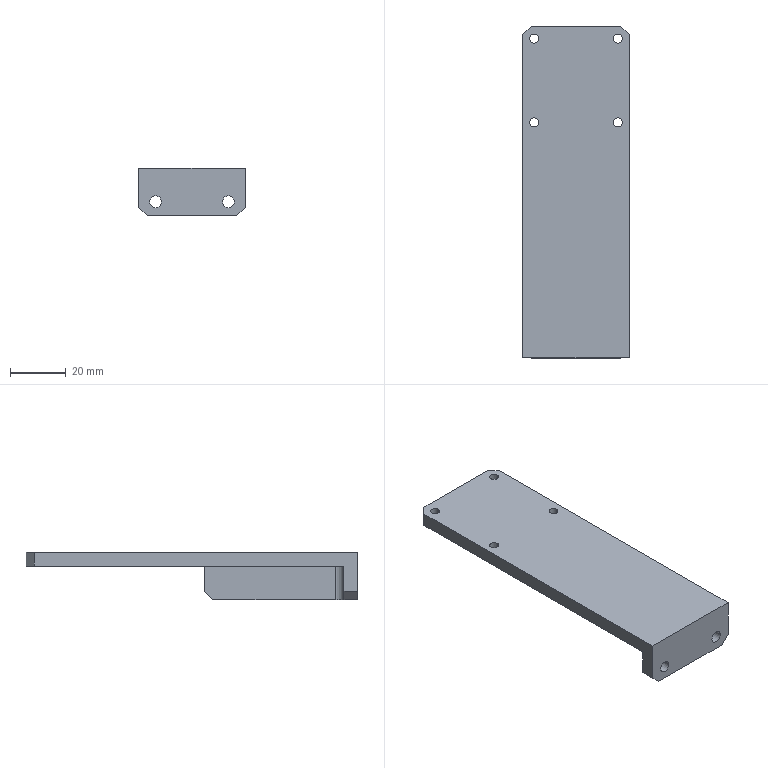Part | NX | 1 solid | 31 faces | box 38.1 x 118.8 x 17 mm | volume 29338 mm3 | plane 17 | cylinder 14 | commonest cylinder face diameters 3.2 x8 4.2 x4 6 x2
STEP:
#1=CARTESIAN_POINT('',(-13.4,24.9,-5.));
#2=VERTEX_POINT('',#1);
#3=CARTESIAN_POINT('',(-16.6,24.9,-5.));
#4=VERTEX_POINT('',#3);
#5=CARTESIAN_POINT('',(-15.,24.9,-5.));
#6=DIRECTION('',(0.,0.,-1.));
#7=DIRECTION('',(-1.,0.,0.));
#8=AXIS2_PLACEMENT_3D('',#5,#6,#7);
#9=CIRCLE('',#8,1.6);
#10=EDGE_CURVE('',#2,#4,#9,.T.);
#11=ORIENTED_EDGE('',*,*,#10,.T.);
#12=CARTESIAN_POINT('',(-16.6,24.9,0.));
#13=VERTEX_POINT('',#12);
#14=CARTESIAN_POINT('',(-16.6,24.9,-17.));
#15=DIRECTION('',(0.,0.,1.));
#16=VECTOR('',#15,1000.);
#17=LINE('',#14,#16);
#18=EDGE_CURVE('',#4,#13,#17,.T.);
#19=ORIENTED_EDGE('',*,*,#18,.T.);
#20=CARTESIAN_POINT('',(-13.4,24.9,0.));
#21=VERTEX_POINT('',#20);
#22=CARTESIAN_POINT('',(-15.,24.9,0.));
#23=DIRECTION('',(0.,0.,1.));
#24=DIRECTION('',(1.,0.,0.));
#25=AXIS2_PLACEMENT_3D('',#22,#23,#24);
#26=CIRCLE('',#25,1.6);
#27=EDGE_CURVE('',#13,#21,#26,.T.);
#28=ORIENTED_EDGE('',*,*,#27,.T.);
#29=CARTESIAN_POINT('',(-13.4,24.9,-17.));
#30=DIRECTION('',(0.,0.,1.));
#31=VECTOR('',#30,1000.);
#32=LINE('',#29,#31);
#33=EDGE_CURVE('',#2,#21,#32,.T.);
#34=ORIENTED_EDGE('',*,*,#33,.F.);
#35=EDGE_LOOP('',(#11,#19,#28,#34));
#36=FACE_BOUND('',#35,.T.);
#37=CARTESIAN_POINT('',(-15.,24.9,-17.));
#38=DIRECTION('',(0.,0.,1.));
#39=DIRECTION('',(-1.,0.,0.));
#40=AXIS2_PLACEMENT_3D('',#37,#38,#39);
#41=CYLINDRICAL_SURFACE('',#40,1.6);
#42=ADVANCED_FACE('',(#36),#41,.F.);
#43=CARTESIAN_POINT('',(16.6,24.9,-5.));
#44=VERTEX_POINT('',#43);
#45=CARTESIAN_POINT('',(13.4,24.9,-5.));
#46=VERTEX_POINT('',#45);
#47=CARTESIAN_POINT('',(15.,24.9,-5.));
#48=DIRECTION('',(0.,0.,-1.));
#49=DIRECTION('',(-1.,0.,0.));
#50=AXIS2_PLACEMENT_3D('',#47,#48,#49);
#51=CIRCLE('',#50,1.6);
#52=EDGE_CURVE('',#44,#46,#51,.T.);
#53=ORIENTED_EDGE('',*,*,#52,.T.);
#54=CARTESIAN_POINT('',(13.4,24.9,0.));
#55=VERTEX_POINT('',#54);
#56=CARTESIAN_POINT('',(13.4,24.9,-17.));
#57=DIRECTION('',(0.,0.,1.));
#58=VECTOR('',#57,1000.);
#59=LINE('',#56,#58);
#60=EDGE_CURVE('',#46,#55,#59,.T.);
#61=ORIENTED_EDGE('',*,*,#60,.T.);
#62=CARTESIAN_POINT('',(16.6,24.9,0.));
#63=VERTEX_POINT('',#62);
#64=CARTESIAN_POINT('',(15.,24.9,0.));
#65=DIRECTION('',(0.,0.,1.));
#66=DIRECTION('',(1.,0.,0.));
#67=AXIS2_PLACEMENT_3D('',#64,#65,#66);
#68=CIRCLE('',#67,1.6);
#69=EDGE_CURVE('',#55,#63,#68,.T.);
#70=ORIENTED_EDGE('',*,*,#69,.T.);
#71=CARTESIAN_POINT('',(16.6,24.9,-17.));
#72=DIRECTION('',(0.,0.,1.));
#73=VECTOR('',#72,1000.);
#74=LINE('',#71,#73);
#75=EDGE_CURVE('',#44,#63,#74,.T.);
#76=ORIENTED_EDGE('',*,*,#75,.F.);
#77=EDGE_LOOP('',(#53,#61,#70,#76));
#78=FACE_BOUND('',#77,.T.);
#79=CARTESIAN_POINT('',(15.,24.9,-17.));
#80=DIRECTION('',(0.,0.,1.));
#81=DIRECTION('',(-1.,0.,0.));
#82=AXIS2_PLACEMENT_3D('',#79,#80,#81);
#83=CYLINDRICAL_SURFACE('',#82,1.6);
#84=ADVANCED_FACE('',(#78),#83,.F.);
#85=CARTESIAN_POINT('',(16.6,54.9,-5.));
#86=VERTEX_POINT('',#85);
#87=CARTESIAN_POINT('',(13.4,54.9,-5.));
#88=VERTEX_POINT('',#87);
#89=CARTESIAN_POINT('',(15.,54.9,-5.));
#90=DIRECTION('',(0.,0.,-1.));
#91=DIRECTION('',(-1.,0.,0.));
#92=AXIS2_PLACEMENT_3D('',#89,#90,#91);
#93=CIRCLE('',#92,1.6);
#94=EDGE_CURVE('',#86,#88,#93,.T.);
#95=ORIENTED_EDGE('',*,*,#94,.T.);
#96=CARTESIAN_POINT('',(13.4,54.9,0.));
#97=VERTEX_POINT('',#96);
#98=CARTESIAN_POINT('',(13.4,54.9,-17.));
#99=DIRECTION('',(0.,0.,1.));
#100=VECTOR('',#99,1000.);
#101=LINE('',#98,#100);
#102=EDGE_CURVE('',#88,#97,#101,.T.);
#103=ORIENTED_EDGE('',*,*,#102,.T.);
#104=CARTESIAN_POINT('',(16.6,54.9,0.));
#105=VERTEX_POINT('',#104);
#106=CARTESIAN_POINT('',(15.,54.9,0.));
#107=DIRECTION('',(0.,0.,1.));
#108=DIRECTION('',(1.,0.,0.));
#109=AXIS2_PLACEMENT_3D('',#106,#107,#108);
#110=CIRCLE('',#109,1.6);
#111=EDGE_CURVE('',#97,#105,#110,.T.);
#112=ORIENTED_EDGE('',*,*,#111,.T.);
#113=CARTESIAN_POINT('',(16.6,54.9,-17.));
#114=DIRECTION('',(0.,0.,1.));
#115=VECTOR('',#114,1000.);
#116=LINE('',#113,#115);
#117=EDGE_CURVE('',#86,#105,#116,.T.);
#118=ORIENTED_EDGE('',*,*,#117,.F.);
#119=EDGE_LOOP('',(#95,#103,#112,#118));
#120=FACE_BOUND('',#119,.T.);
#121=CARTESIAN_POINT('',(15.,54.9,-17.));
#122=DIRECTION('',(0.,0.,1.));
#123=DIRECTION('',(-1.,0.,0.));
#124=AXIS2_PLACEMENT_3D('',#121,#122,#123);
#125=CYLINDRICAL_SURFACE('',#124,1.6);
#126=ADVANCED_FACE('',(#120),#125,.F.);
#127=CARTESIAN_POINT('',(-13.4,54.9,-5.));
#128=VERTEX_POINT('',#127);
#129=CARTESIAN_POINT('',(-16.6,54.9,-5.));
#130=VERTEX_POINT('',#129);
#131=CARTESIAN_POINT('',(-15.,54.9,-5.));
#132=DIRECTION('',(0.,0.,-1.));
#133=DIRECTION('',(-1.,0.,0.));
#134=AXIS2_PLACEMENT_3D('',#131,#132,#133);
#135=CIRCLE('',#134,1.6);
#136=EDGE_CURVE('',#128,#130,#135,.T.);
#137=ORIENTED_EDGE('',*,*,#136,.T.);
#138=CARTESIAN_POINT('',(-16.6,54.9,0.));
#139=VERTEX_POINT('',#138);
#140=CARTESIAN_POINT('',(-16.6,54.9,-17.));
#141=DIRECTION('',(0.,0.,1.));
#142=VECTOR('',#141,1000.);
#143=LINE('',#140,#142);
#144=EDGE_CURVE('',#130,#139,#143,.T.);
#145=ORIENTED_EDGE('',*,*,#144,.T.);
#146=CARTESIAN_POINT('',(-13.4,54.9,0.));
#147=VERTEX_POINT('',#146);
#148=CARTESIAN_POINT('',(-15.,54.9,0.));
#149=DIRECTION('',(0.,0.,1.));
#150=DIRECTION('',(1.,0.,0.));
#151=AXIS2_PLACEMENT_3D('',#148,#149,#150);
#152=CIRCLE('',#151,1.6);
#153=EDGE_CURVE('',#139,#147,#152,.T.);
#154=ORIENTED_EDGE('',*,*,#153,.T.);
#155=CARTESIAN_POINT('',(-13.4,54.9,-17.));
#156=DIRECTION('',(0.,0.,1.));
#157=VECTOR('',#156,1000.);
#158=LINE('',#155,#157);
#159=EDGE_CURVE('',#128,#147,#158,.T.);
#160=ORIENTED_EDGE('',*,*,#159,.F.);
#161=EDGE_LOOP('',(#137,#145,#154,#160));
#162=FACE_BOUND('',#161,.T.);
#163=CARTESIAN_POINT('',(-15.,54.9,-17.));
#164=DIRECTION('',(0.,0.,1.));
#165=DIRECTION('',(-1.,0.,0.));
#166=AXIS2_PLACEMENT_3D('',#163,#164,#165);
#167=CYLINDRICAL_SURFACE('',#166,1.6);
#168=ADVANCED_FACE('',(#162),#167,.F.);
#169=CARTESIAN_POINT('',(-10.9,-59.4,-12.));
#170=VERTEX_POINT('',#169);
#171=CARTESIAN_POINT('',(-15.1,-59.4,-12.));
#172=VERTEX_POINT('',#171);
#173=CARTESIAN_POINT('',(-13.,-59.4,-12.));
#174=DIRECTION('',(0.,1.,0.));
#175=DIRECTION('',(-1.,0.,0.));
#176=AXIS2_PLACEMENT_3D('',#173,#174,#175);
#177=CIRCLE('',#176,2.1);
#178=EDGE_CURVE('',#170,#172,#177,.T.);
#179=ORIENTED_EDGE('',*,*,#178,.F.);
#180=CARTESIAN_POINT('',(-10.9,-54.4,-12.));
#181=VERTEX_POINT('',#180);
#182=CARTESIAN_POINT('',(-10.9,-59.4,-12.));
#183=DIRECTION('',(0.,1.,0.));
#184=VECTOR('',#183,1000.);
#185=LINE('',#182,#184);
#186=EDGE_CURVE('',#170,#181,#185,.T.);
#187=ORIENTED_EDGE('',*,*,#186,.T.);
#188=CARTESIAN_POINT('',(-15.1,-54.4,-12.));
#189=VERTEX_POINT('',#188);
#190=CARTESIAN_POINT('',(-13.,-54.4,-12.));
#191=DIRECTION('',(0.,1.,0.));
#192=DIRECTION('',(-1.,0.,0.));
#193=AXIS2_PLACEMENT_3D('',#190,#191,#192);
#194=CIRCLE('',#193,2.1);
#195=EDGE_CURVE('',#181,#189,#194,.T.);
#196=ORIENTED_EDGE('',*,*,#195,.T.);
#197=CARTESIAN_POINT('',(-15.1,-59.4,-12.));
#198=DIRECTION('',(0.,1.,0.));
#199=VECTOR('',#198,1000.);
#200=LINE('',#197,#199);
#201=EDGE_CURVE('',#172,#189,#200,.T.);
#202=ORIENTED_EDGE('',*,*,#201,.F.);
#203=EDGE_LOOP('',(#179,#187,#196,#202));
#204=FACE_BOUND('',#203,.T.);
#205=CARTESIAN_POINT('',(-13.,-59.4,-12.));
#206=DIRECTION('',(0.,1.,0.));
#207=DIRECTION('',(1.,0.,0.));
#208=AXIS2_PLACEMENT_3D('',#205,#206,#207);
#209=CYLINDRICAL_SURFACE('',#208,2.1);
#210=ADVANCED_FACE('',(#204),#209,.F.);
#211=CARTESIAN_POINT('',(15.1,-59.4,-12.));
#212=VERTEX_POINT('',#211);
#213=CARTESIAN_POINT('',(10.9,-59.4,-12.));
#214=VERTEX_POINT('',#213);
#215=CARTESIAN_POINT('',(13.,-59.4,-12.));
#216=DIRECTION('',(0.,1.,0.));
#217=DIRECTION('',(-1.,0.,0.));
#218=AXIS2_PLACEMENT_3D('',#215,#216,#217);
#219=CIRCLE('',#218,2.1);
#220=EDGE_CURVE('',#212,#214,#219,.T.);
#221=ORIENTED_EDGE('',*,*,#220,.F.);
#222=CARTESIAN_POINT('',(15.1,-54.4,-12.));
#223=VERTEX_POINT('',#222);
#224=CARTESIAN_POINT('',(15.1,-59.4,-12.));
#225=DIRECTION('',(0.,1.,0.));
#226=VECTOR('',#225,1000.);
#227=LINE('',#224,#226);
#228=EDGE_CURVE('',#212,#223,#227,.T.);
#229=ORIENTED_EDGE('',*,*,#228,.T.);
#230=CARTESIAN_POINT('',(10.9,-54.4,-12.));
#231=VERTEX_POINT('',#230);
#232=CARTESIAN_POINT('',(13.,-54.4,-12.));
#233=DIRECTION('',(0.,1.,0.));
#234=DIRECTION('',(-1.,0.,0.));
#235=AXIS2_PLACEMENT_3D('',#232,#233,#234);
#236=CIRCLE('',#235,2.1);
#237=EDGE_CURVE('',#223,#231,#236,.T.);
#238=ORIENTED_EDGE('',*,*,#237,.T.);
#239=CARTESIAN_POINT('',(10.9,-59.4,-12.));
#240=DIRECTION('',(0.,1.,0.));
#241=VECTOR('',#240,1000.);
#242=LINE('',#239,#241);
#243=EDGE_CURVE('',#214,#231,#242,.T.);
#244=ORIENTED_EDGE('',*,*,#243,.F.);
#245=EDGE_LOOP('',(#221,#229,#238,#244));
#246=FACE_BOUND('',#245,.T.);
#247=CARTESIAN_POINT('',(13.,-59.4,-12.));
#248=DIRECTION('',(0.,1.,0.));
#249=DIRECTION('',(1.,0.,0.));
#250=AXIS2_PLACEMENT_3D('',#247,#248,#249);
#251=CYLINDRICAL_SURFACE('',#250,2.1);
#252=ADVANCED_FACE('',(#246),#251,.F.);
#253=ORIENTED_EDGE('',*,*,#10,.F.);
#254=CARTESIAN_POINT('',(-15.,24.9,-5.));
#255=DIRECTION('',(0.,0.,-1.));
#256=DIRECTION('',(-1.,0.,0.));
#257=AXIS2_PLACEMENT_3D('',#254,#255,#256);
#258=CIRCLE('',#257,1.6);
#259=EDGE_CURVE('',#4,#2,#258,.T.);
#260=ORIENTED_EDGE('',*,*,#259,.F.);
#261=EDGE_LOOP('',(#253,#260));
#262=FACE_BOUND('',#261,.T.);
#263=ORIENTED_EDGE('',*,*,#52,.F.);
#264=CARTESIAN_POINT('',(15.,24.9,-5.));
#265=DIRECTION('',(0.,0.,-1.));
#266=DIRECTION('',(-1.,0.,0.));
#267=AXIS2_PLACEMENT_3D('',#264,#265,#266);
#268=CIRCLE('',#267,1.6);
#269=EDGE_CURVE('',#46,#44,#268,.T.);
#270=ORIENTED_EDGE('',*,*,#269,.F.);
#271=EDGE_LOOP('',(#263,#270));
#272=FACE_BOUND('',#271,.T.);
#273=ORIENTED_EDGE('',*,*,#94,.F.);
#274=CARTESIAN_POINT('',(15.,54.9,-5.));
#275=DIRECTION('',(0.,0.,-1.));
#276=DIRECTION('',(-1.,0.,0.));
#277=AXIS2_PLACEMENT_3D('',#274,#275,#276);
#278=CIRCLE('',#277,1.6);
#279=EDGE_CURVE('',#88,#86,#278,.T.);
#280=ORIENTED_EDGE('',*,*,#279,.F.);
#281=EDGE_LOOP('',(#273,#280));
#282=FACE_BOUND('',#281,.T.);
#283=ORIENTED_EDGE('',*,*,#136,.F.);
#284=CARTESIAN_POINT('',(-15.,54.9,-5.));
#285=DIRECTION('',(0.,0.,-1.));
#286=DIRECTION('',(-1.,0.,0.));
#287=AXIS2_PLACEMENT_3D('',#284,#285,#286);
#288=CIRCLE('',#287,1.6);
#289=EDGE_CURVE('',#130,#128,#288,.T.);
#290=ORIENTED_EDGE('',*,*,#289,.F.);
#291=EDGE_LOOP('',(#283,#290));
#292=FACE_BOUND('',#291,.T.);
#293=CARTESIAN_POINT('',(-4.,-51.4,-5.));
#294=VERTEX_POINT('',#293);
#295=CARTESIAN_POINT('',(-4.,-4.4,-5.));
#296=VERTEX_POINT('',#295);
#297=CARTESIAN_POINT('',(-4.,-54.4,-5.));
#298=DIRECTION('',(0.,1.,0.));
#299=VECTOR('',#298,1000.);
#300=LINE('',#297,#299);
#301=EDGE_CURVE('',#294,#296,#300,.T.);
#302=ORIENTED_EDGE('',*,*,#301,.F.);
#303=CARTESIAN_POINT('',(-7.,-54.4,-5.));
#304=VERTEX_POINT('',#303);
#305=CARTESIAN_POINT('',(-7.,-51.4,-5.));
#306=DIRECTION('',(0.,0.,-1.));
#307=DIRECTION('',(-1.,0.,0.));
#308=AXIS2_PLACEMENT_3D('',#305,#306,#307);
#309=CIRCLE('',#308,3.);
#310=EDGE_CURVE('',#294,#304,#309,.T.);
#311=ORIENTED_EDGE('',*,*,#310,.T.);
#312=CARTESIAN_POINT('',(-19.05,-54.4,-5.));
#313=VERTEX_POINT('',#312);
#314=CARTESIAN_POINT('',(-19.05,-54.4,-5.));
#315=DIRECTION('',(1.,0.,0.));
#316=VECTOR('',#315,1000.);
#317=LINE('',#314,#316);
#318=EDGE_CURVE('',#313,#304,#317,.T.);
#319=ORIENTED_EDGE('',*,*,#318,.F.);
#320=CARTESIAN_POINT('',(-19.05,56.4,-5.));
#321=VERTEX_POINT('',#320);
#322=CARTESIAN_POINT('',(-19.05,-59.4,-5.));
#323=DIRECTION('',(0.,-1.,0.));
#324=VECTOR('',#323,1000.);
#325=LINE('',#322,#324);
#326=EDGE_CURVE('',#321,#313,#325,.T.);
#327=ORIENTED_EDGE('',*,*,#326,.F.);
#328=CARTESIAN_POINT('',(-16.05,59.4,-5.));
#329=VERTEX_POINT('',#328);
#330=CARTESIAN_POINT('',(-76.95,-1.5,-5.));
#331=DIRECTION('',(0.7071,0.7071,0.));
#332=VECTOR('',#331,1000.);
#333=LINE('',#330,#332);
#334=EDGE_CURVE('',#321,#329,#333,.T.);
#335=ORIENTED_EDGE('',*,*,#334,.T.);
#336=CARTESIAN_POINT('',(16.05,59.4,-5.));
#337=VERTEX_POINT('',#336);
#338=CARTESIAN_POINT('',(-19.05,59.4,-5.));
#339=DIRECTION('',(-1.,0.,0.));
#340=VECTOR('',#339,1000.);
#341=LINE('',#338,#340);
#342=EDGE_CURVE('',#337,#329,#341,.T.);
#343=ORIENTED_EDGE('',*,*,#342,.F.);
#344=CARTESIAN_POINT('',(19.05,56.4,-5.));
#345=VERTEX_POINT('',#344);
#346=CARTESIAN_POINT('',(57.9,17.55,-5.));
#347=DIRECTION('',(0.7071,-0.7071,0.));
#348=VECTOR('',#347,1000.);
#349=LINE('',#346,#348);
#350=EDGE_CURVE('',#337,#345,#349,.T.);
#351=ORIENTED_EDGE('',*,*,#350,.T.);
#352=CARTESIAN_POINT('',(19.05,-54.4,-5.));
#353=VERTEX_POINT('',#352);
#354=CARTESIAN_POINT('',(19.05,-59.4,-5.));
#355=DIRECTION('',(0.,1.,0.));
#356=VECTOR('',#355,1000.);
#357=LINE('',#354,#356);
#358=EDGE_CURVE('',#353,#345,#357,.T.);
#359=ORIENTED_EDGE('',*,*,#358,.F.);
#360=CARTESIAN_POINT('',(7.,-54.4,-5.));
#361=VERTEX_POINT('',#360);
#362=CARTESIAN_POINT('',(-19.05,-54.4,-5.));
#363=DIRECTION('',(1.,0.,0.));
#364=VECTOR('',#363,1000.);
#365=LINE('',#362,#364);
#366=EDGE_CURVE('',#361,#353,#365,.T.);
#367=ORIENTED_EDGE('',*,*,#366,.F.);
#368=CARTESIAN_POINT('',(4.,-51.4,-5.));
#369=VERTEX_POINT('',#368);
#370=CARTESIAN_POINT('',(7.,-51.4,-5.));
#371=DIRECTION('',(0.,0.,-1.));
#372=DIRECTION('',(-1.,0.,0.));
#373=AXIS2_PLACEMENT_3D('',#370,#371,#372);
#374=CIRCLE('',#373,3.);
#375=EDGE_CURVE('',#361,#369,#374,.T.);
#376=ORIENTED_EDGE('',*,*,#375,.T.);
#377=CARTESIAN_POINT('',(4.,-4.4,-5.));
#378=VERTEX_POINT('',#377);
#379=CARTESIAN_POINT('',(4.,-54.4,-5.));
#380=DIRECTION('',(0.,-1.,0.));
#381=VECTOR('',#380,1000.);
#382=LINE('',#379,#381);
#383=EDGE_CURVE('',#378,#369,#382,.T.);
#384=ORIENTED_EDGE('',*,*,#383,.F.);
#385=CARTESIAN_POINT('',(4.,-4.4,-5.));
#386=DIRECTION('',(1.,0.,0.));
#387=VECTOR('',#386,1000.);
#388=LINE('',#385,#387);
#389=EDGE_CURVE('',#296,#378,#388,.T.);
#390=ORIENTED_EDGE('',*,*,#389,.F.);
#391=EDGE_LOOP('',(#302,#311,#319,#327,#335,#343,#351,#359,#367,#376,#384,#390));
#392=FACE_BOUND('',#391,.T.);
#393=CARTESIAN_POINT('',(-19.05,-59.4,-5.));
#394=DIRECTION('',(0.,0.,-1.));
#395=DIRECTION('',(1.,0.,0.));
#396=AXIS2_PLACEMENT_3D('',#393,#394,#395);
#397=PLANE('',#396);
#398=ADVANCED_FACE('',(#262,#272,#282,#292,#392),#397,.T.);
#399=CARTESIAN_POINT('',(13.,-54.4,-12.));
#400=DIRECTION('',(0.,1.,0.));
#401=DIRECTION('',(-1.,0.,0.));
#402=AXIS2_PLACEMENT_3D('',#399,#400,#401);
#403=CIRCLE('',#402,2.1);
#404=EDGE_CURVE('',#231,#223,#403,.T.);
#405=ORIENTED_EDGE('',*,*,#404,.F.);
#406=ORIENTED_EDGE('',*,*,#237,.F.);
#407=EDGE_LOOP('',(#405,#406));
#408=FACE_BOUND('',#407,.T.);
#409=CARTESIAN_POINT('',(7.,-54.4,-17.));
#410=VERTEX_POINT('',#409);
#411=CARTESIAN_POINT('',(16.05,-54.4,-17.));
#412=VERTEX_POINT('',#411);
#413=CARTESIAN_POINT('',(-19.05,-54.4,-17.));
#414=DIRECTION('',(1.,0.,0.));
#415=VECTOR('',#414,1000.);
#416=LINE('',#413,#415);
#417=EDGE_CURVE('',#410,#412,#416,.T.);
#418=ORIENTED_EDGE('',*,*,#417,.F.);
#419=CARTESIAN_POINT('',(7.,-54.4,-5.));
#420=DIRECTION('',(0.,0.,1.));
#421=VECTOR('',#420,1000.);
#422=LINE('',#419,#421);
#423=EDGE_CURVE('',#410,#361,#422,.T.);
#424=ORIENTED_EDGE('',*,*,#423,.T.);
#425=ORIENTED_EDGE('',*,*,#366,.T.);
#426=CARTESIAN_POINT('',(19.05,-54.4,-14.));
#427=VERTEX_POINT('',#426);
#428=CARTESIAN_POINT('',(19.05,-54.4,-17.));
#429=DIRECTION('',(0.,0.,1.));
#430=VECTOR('',#429,1000.);
#431=LINE('',#428,#430);
#432=EDGE_CURVE('',#427,#353,#431,.T.);
#433=ORIENTED_EDGE('',*,*,#432,.F.);
#434=CARTESIAN_POINT('',(16.05,-54.4,-17.));
#435=DIRECTION('',(-0.7071,0.,-0.7071));
#436=VECTOR('',#435,1000.);
#437=LINE('',#434,#436);
#438=EDGE_CURVE('',#427,#412,#437,.T.);
#439=ORIENTED_EDGE('',*,*,#438,.T.);
#440=EDGE_LOOP('',(#418,#424,#425,#433,#439));
#441=FACE_BOUND('',#440,.T.);
#442=CARTESIAN_POINT('',(-19.05,-54.4,-17.));
#443=DIRECTION('',(0.,-1.,0.));
#444=DIRECTION('',(-1.,0.,0.));
#445=AXIS2_PLACEMENT_3D('',#442,#443,#444);
#446=PLANE('',#445);
#447=ADVANCED_FACE('',(#408,#441),#446,.F.);
#448=CARTESIAN_POINT('',(-13.,-54.4,-12.));
#449=DIRECTION('',(0.,1.,0.));
#450=DIRECTION('',(-1.,0.,0.));
#451=AXIS2_PLACEMENT_3D('',#448,#449,#450);
#452=CIRCLE('',#451,2.1);
#453=EDGE_CURVE('',#189,#181,#452,.T.);
#454=ORIENTED_EDGE('',*,*,#453,.F.);
#455=ORIENTED_EDGE('',*,*,#195,.F.);
#456=EDGE_LOOP('',(#454,#455));
#457=FACE_BOUND('',#456,.T.);
#458=ORIENTED_EDGE('',*,*,#318,.T.);
#459=CARTESIAN_POINT('',(-7.,-54.4,-17.));
#460=VERTEX_POINT('',#459);
#461=CARTESIAN_POINT('',(-7.,-54.4,-17.));
#462=DIRECTION('',(0.,0.,-1.));
#463=VECTOR('',#462,1000.);
#464=LINE('',#461,#463);
#465=EDGE_CURVE('',#304,#460,#464,.T.);
#466=ORIENTED_EDGE('',*,*,#465,.T.);
#467=CARTESIAN_POINT('',(-16.05,-54.4,-17.));
#468=VERTEX_POINT('',#467);
#469=CARTESIAN_POINT('',(-19.05,-54.4,-17.));
#470=DIRECTION('',(1.,0.,0.));
#471=VECTOR('',#470,1000.);
#472=LINE('',#469,#471);
#473=EDGE_CURVE('',#468,#460,#472,.T.);
#474=ORIENTED_EDGE('',*,*,#473,.F.);
#475=CARTESIAN_POINT('',(-19.05,-54.4,-14.));
#476=VERTEX_POINT('',#475);
#477=CARTESIAN_POINT('',(-16.05,-54.4,-17.));
#478=DIRECTION('',(-0.7071,0.,0.7071));
#479=VECTOR('',#478,1000.);
#480=LINE('',#477,#479);
#481=EDGE_CURVE('',#468,#476,#480,.T.);
#482=ORIENTED_EDGE('',*,*,#481,.T.);
#483=CARTESIAN_POINT('',(-19.05,-54.4,-17.));
#484=DIRECTION('',(0.,0.,1.));
#485=VECTOR('',#484,1000.);
#486=LINE('',#483,#485);
#487=EDGE_CURVE('',#476,#313,#486,.T.);
#488=ORIENTED_EDGE('',*,*,#487,.T.);
#489=EDGE_LOOP('',(#458,#466,#474,#482,#488));
#490=FACE_BOUND('',#489,.T.);
#491=CARTESIAN_POINT('',(-19.05,-54.4,-17.));
#492=DIRECTION('',(0.,-1.,0.));
#493=DIRECTION('',(-1.,0.,0.));
#494=AXIS2_PLACEMENT_3D('',#491,#492,#493);
#495=PLANE('',#494);
#496=ADVANCED_FACE('',(#457,#490),#495,.F.);
#497=ORIENTED_EDGE('',*,*,#487,.F.);
#498=CARTESIAN_POINT('',(-19.05,-59.4,-14.));
#499=VERTEX_POINT('',#498);
#500=CARTESIAN_POINT('',(-19.05,-59.4,-14.));
#501=DIRECTION('',(0.,-1.,0.));
#502=VECTOR('',#501,1000.);
#503=LINE('',#500,#502);
#504=EDGE_CURVE('',#476,#499,#503,.T.);
#505=ORIENTED_EDGE('',*,*,#504,.T.);
#506=CARTESIAN_POINT('',(-19.05,-59.4,0.));
#507=VERTEX_POINT('',#506);
#508=CARTESIAN_POINT('',(-19.05,-59.4,0.));
#509=DIRECTION('',(0.,0.,-1.));
#510=VECTOR('',#509,1000.);
#511=LINE('',#508,#510);
#512=EDGE_CURVE('',#507,#499,#511,.T.);
#513=ORIENTED_EDGE('',*,*,#512,.F.);
#514=CARTESIAN_POINT('',(-19.05,56.4,0.));
#515=VERTEX_POINT('',#514);
#516=CARTESIAN_POINT('',(-19.05,-59.4,0.));
#517=DIRECTION('',(0.,-1.,0.));
#518=VECTOR('',#517,1000.);
#519=LINE('',#516,#518);
#520=EDGE_CURVE('',#515,#507,#519,.T.);
#521=ORIENTED_EDGE('',*,*,#520,.F.);
#522=CARTESIAN_POINT('',(-19.05,56.4,0.));
#523=DIRECTION('',(0.,0.,-1.));
#524=VECTOR('',#523,1000.);
#525=LINE('',#522,#524);
#526=EDGE_CURVE('',#515,#321,#525,.T.);
#527=ORIENTED_EDGE('',*,*,#526,.T.);
#528=ORIENTED_EDGE('',*,*,#326,.T.);
#529=EDGE_LOOP('',(#497,#505,#513,#521,#527,#528));
#530=FACE_BOUND('',#529,.T.);
#531=CARTESIAN_POINT('',(-19.05,-59.4,0.));
#532=DIRECTION('',(1.,0.,0.));
#533=DIRECTION('',(0.,-1.,0.));
#534=AXIS2_PLACEMENT_3D('',#531,#532,#533);
#535=PLANE('',#534);
#536=ADVANCED_FACE('',(#530),#535,.F.);
#537=CARTESIAN_POINT('',(-13.,-59.4,-12.));
#538=DIRECTION('',(0.,1.,0.));
#539=DIRECTION('',(-1.,0.,0.));
#540=AXIS2_PLACEMENT_3D('',#537,#538,#539);
#541=CIRCLE('',#540,2.1);
#542=EDGE_CURVE('',#172,#170,#541,.T.);
#543=ORIENTED_EDGE('',*,*,#542,.T.);
#544=ORIENTED_EDGE('',*,*,#178,.T.);
#545=EDGE_LOOP('',(#543,#544));
#546=FACE_BOUND('',#545,.T.);
#547=CARTESIAN_POINT('',(13.,-59.4,-12.));
#548=DIRECTION('',(0.,1.,0.));
#549=DIRECTION('',(-1.,0.,0.));
#550=AXIS2_PLACEMENT_3D('',#547,#548,#549);
#551=CIRCLE('',#550,2.1);
#552=EDGE_CURVE('',#214,#212,#551,.T.);
#553=ORIENTED_EDGE('',*,*,#552,.T.);
#554=ORIENTED_EDGE('',*,*,#220,.T.);
#555=EDGE_LOOP('',(#553,#554));
#556=FACE_BOUND('',#555,.T.);
#557=CARTESIAN_POINT('',(16.05,-59.4,-17.));
#558=VERTEX_POINT('',#557);
#559=CARTESIAN_POINT('',(-16.05,-59.4,-17.));
#560=VERTEX_POINT('',#559);
#561=CARTESIAN_POINT('',(-19.05,-59.4,-17.));
#562=DIRECTION('',(-1.,0.,0.));
#563=VECTOR('',#562,1000.);
#564=LINE('',#561,#563);
#565=EDGE_CURVE('',#558,#560,#564,.T.);
#566=ORIENTED_EDGE('',*,*,#565,.F.);
#567=CARTESIAN_POINT('',(19.05,-59.4,-14.));
#568=VERTEX_POINT('',#567);
#569=CARTESIAN_POINT('',(16.05,-59.4,-17.));
#570=DIRECTION('',(0.7071,0.,0.7071));
#571=VECTOR('',#570,1000.);
#572=LINE('',#569,#571);
#573=EDGE_CURVE('',#558,#568,#572,.T.);
#574=ORIENTED_EDGE('',*,*,#573,.T.);
#575=CARTESIAN_POINT('',(19.05,-59.4,0.));
#576=VERTEX_POINT('',#575);
#577=CARTESIAN_POINT('',(19.05,-59.4,0.));
#578=DIRECTION('',(0.,0.,-1.));
#579=VECTOR('',#578,1000.);
#580=LINE('',#577,#579);
#581=EDGE_CURVE('',#576,#568,#580,.T.);
#582=ORIENTED_EDGE('',*,*,#581,.F.);
#583=CARTESIAN_POINT('',(-19.05,-59.4,0.));
#584=DIRECTION('',(1.,0.,0.));
#585=VECTOR('',#584,1000.);
#586=LINE('',#583,#585);
#587=EDGE_CURVE('',#507,#576,#586,.T.);
#588=ORIENTED_EDGE('',*,*,#587,.F.);
#589=ORIENTED_EDGE('',*,*,#512,.T.);
#590=CARTESIAN_POINT('',(-16.05,-59.4,-17.));
#591=DIRECTION('',(0.7071,0.,-0.7071));
#592=VECTOR('',#591,1000.);
#593=LINE('',#590,#592);
#594=EDGE_CURVE('',#499,#560,#593,.T.);
#595=ORIENTED_EDGE('',*,*,#594,.T.);
#596=EDGE_LOOP('',(#566,#574,#582,#588,#589,#595));
#597=FACE_BOUND('',#596,.T.);
#598=CARTESIAN_POINT('',(-19.05,-59.4,0.));
#599=DIRECTION('',(0.,1.,0.));
#600=DIRECTION('',(0.,0.,-1.));
#601=AXIS2_PLACEMENT_3D('',#598,#599,#600);
#602=PLANE('',#601);
#603=ADVANCED_FACE('',(#546,#556,#597),#602,.F.);
#604=ORIENTED_EDGE('',*,*,#581,.T.);
#605=CARTESIAN_POINT('',(19.05,-54.4,-14.));
#606=DIRECTION('',(0.,1.,0.));
#607=VECTOR('',#606,1000.);
#608=LINE('',#605,#607);
#609=EDGE_CURVE('',#568,#427,#608,.T.);
#610=ORIENTED_EDGE('',*,*,#609,.T.);
#611=ORIENTED_EDGE('',*,*,#432,.T.);
#612=ORIENTED_EDGE('',*,*,#358,.T.);
#613=CARTESIAN_POINT('',(19.05,56.4,0.));
#614=VERTEX_POINT('',#613);
#615=CARTESIAN_POINT('',(19.05,56.4,0.));
#616=DIRECTION('',(0.,0.,1.));
#617=VECTOR('',#616,1000.);
#618=LINE('',#615,#617);
#619=EDGE_CURVE('',#345,#614,#618,.T.);
#620=ORIENTED_EDGE('',*,*,#619,.T.);
#621=CARTESIAN_POINT('',(19.05,-59.4,0.));
#622=DIRECTION('',(0.,1.,0.));
#623=VECTOR('',#622,1000.);
#624=LINE('',#621,#623);
#625=EDGE_CURVE('',#576,#614,#624,.T.);
#626=ORIENTED_EDGE('',*,*,#625,.F.);
#627=EDGE_LOOP('',(#604,#610,#611,#612,#620,#626));
#628=FACE_BOUND('',#627,.T.);
#629=CARTESIAN_POINT('',(19.05,-59.4,0.));
#630=DIRECTION('',(-1.,0.,0.));
#631=DIRECTION('',(0.,1.,0.));
#632=AXIS2_PLACEMENT_3D('',#629,#630,#631);
#633=PLANE('',#632);
#634=ADVANCED_FACE('',(#628),#633,.F.);
#635=ORIENTED_EDGE('',*,*,#342,.T.);
#636=CARTESIAN_POINT('',(-16.05,59.4,0.));
#637=VERTEX_POINT('',#636);
#638=CARTESIAN_POINT('',(-16.05,59.4,0.));
#639=DIRECTION('',(0.,0.,1.));
#640=VECTOR('',#639,1000.);
#641=LINE('',#638,#640);
#642=EDGE_CURVE('',#329,#637,#641,.T.);
#643=ORIENTED_EDGE('',*,*,#642,.T.);
#644=CARTESIAN_POINT('',(16.05,59.4,0.));
#645=VERTEX_POINT('',#644);
#646=CARTESIAN_POINT('',(-19.05,59.4,0.));
#647=DIRECTION('',(-1.,0.,0.));
#648=VECTOR('',#647,1000.);
#649=LINE('',#646,#648);
#650=EDGE_CURVE('',#645,#637,#649,.T.);
#651=ORIENTED_EDGE('',*,*,#650,.F.);
#652=CARTESIAN_POINT('',(16.05,59.4,0.));
#653=DIRECTION('',(0.,0.,-1.));
#654=VECTOR('',#653,1000.);
#655=LINE('',#652,#654);
#656=EDGE_CURVE('',#645,#337,#655,.T.);
#657=ORIENTED_EDGE('',*,*,#656,.T.);
#658=EDGE_LOOP('',(#635,#643,#651,#657));
#659=FACE_BOUND('',#658,.T.);
#660=CARTESIAN_POINT('',(-19.05,59.4,0.));
#661=DIRECTION('',(0.,-1.,0.));
#662=DIRECTION('',(-1.,0.,0.));
#663=AXIS2_PLACEMENT_3D('',#660,#661,#662);
#664=PLANE('',#663);
#665=ADVANCED_FACE('',(#659),#664,.F.);
#666=CARTESIAN_POINT('',(-15.,24.9,0.));
#667=DIRECTION('',(0.,0.,1.));
#668=DIRECTION('',(1.,0.,0.));
#669=AXIS2_PLACEMENT_3D('',#666,#667,#668);
#670=CIRCLE('',#669,1.6);
#671=EDGE_CURVE('',#21,#13,#670,.T.);
#672=ORIENTED_EDGE('',*,*,#671,.F.);
#673=ORIENTED_EDGE('',*,*,#27,.F.);
#674=EDGE_LOOP('',(#672,#673));
#675=FACE_BOUND('',#674,.T.);
#676=CARTESIAN_POINT('',(15.,24.9,0.));
#677=DIRECTION('',(0.,0.,1.));
#678=DIRECTION('',(1.,0.,0.));
#679=AXIS2_PLACEMENT_3D('',#676,#677,#678);
#680=CIRCLE('',#679,1.6);
#681=EDGE_CURVE('',#63,#55,#680,.T.);
#682=ORIENTED_EDGE('',*,*,#681,.F.);
#683=ORIENTED_EDGE('',*,*,#69,.F.);
#684=EDGE_LOOP('',(#682,#683));
#685=FACE_BOUND('',#684,.T.);
#686=CARTESIAN_POINT('',(15.,54.9,0.));
#687=DIRECTION('',(0.,0.,1.));
#688=DIRECTION('',(1.,0.,0.));
#689=AXIS2_PLACEMENT_3D('',#686,#687,#688);
#690=CIRCLE('',#689,1.6);
#691=EDGE_CURVE('',#105,#97,#690,.T.);
#692=ORIENTED_EDGE('',*,*,#691,.F.);
#693=ORIENTED_EDGE('',*,*,#111,.F.);
#694=EDGE_LOOP('',(#692,#693));
#695=FACE_BOUND('',#694,.T.);
#696=CARTESIAN_POINT('',(-15.,54.9,0.));
#697=DIRECTION('',(0.,0.,1.));
#698=DIRECTION('',(1.,0.,0.));
#699=AXIS2_PLACEMENT_3D('',#696,#697,#698);
#700=CIRCLE('',#699,1.6);
#701=EDGE_CURVE('',#147,#139,#700,.T.);
#702=ORIENTED_EDGE('',*,*,#701,.F.);
#703=ORIENTED_EDGE('',*,*,#153,.F.);
#704=EDGE_LOOP('',(#702,#703));
#705=FACE_BOUND('',#704,.T.);
#706=ORIENTED_EDGE('',*,*,#650,.T.);
#707=CARTESIAN_POINT('',(-19.05,56.4,0.));
#708=DIRECTION('',(-0.7071,-0.7071,0.));
#709=VECTOR('',#708,1000.);
#710=LINE('',#707,#709);
#711=EDGE_CURVE('',#637,#515,#710,.T.);
#712=ORIENTED_EDGE('',*,*,#711,.T.);
#713=ORIENTED_EDGE('',*,*,#520,.T.);
#714=ORIENTED_EDGE('',*,*,#587,.T.);
#715=ORIENTED_EDGE('',*,*,#625,.T.);
#716=CARTESIAN_POINT('',(16.05,59.4,0.));
#717=DIRECTION('',(-0.7071,0.7071,0.));
#718=VECTOR('',#717,1000.);
#719=LINE('',#716,#718);
#720=EDGE_CURVE('',#614,#645,#719,.T.);
#721=ORIENTED_EDGE('',*,*,#720,.T.);
#722=EDGE_LOOP('',(#706,#712,#713,#714,#715,#721));
#723=FACE_BOUND('',#722,.T.);
#724=CARTESIAN_POINT('',(-19.05,-59.4,0.));
#725=DIRECTION('',(0.,0.,-1.));
#726=DIRECTION('',(1.,0.,0.));
#727=AXIS2_PLACEMENT_3D('',#724,#725,#726);
#728=PLANE('',#727);
#729=ADVANCED_FACE('',(#675,#685,#695,#705,#723),#728,.F.);
#730=ORIENTED_EDGE('',*,*,#473,.T.);
#731=CARTESIAN_POINT('',(-4.,-51.4,-17.));
#732=VERTEX_POINT('',#731);
#733=CARTESIAN_POINT('',(-7.,-51.4,-17.));
#734=DIRECTION('',(0.,0.,1.));
#735=DIRECTION('',(-1.,0.,0.));
#736=AXIS2_PLACEMENT_3D('',#733,#734,#735);
#737=CIRCLE('',#736,3.);
#738=EDGE_CURVE('',#460,#732,#737,.T.);
#739=ORIENTED_EDGE('',*,*,#738,.T.);
#740=CARTESIAN_POINT('',(-4.,-7.4,-17.));
#741=VERTEX_POINT('',#740);
#742=CARTESIAN_POINT('',(-4.,-54.4,-17.));
#743=DIRECTION('',(0.,1.,0.));
#744=VECTOR('',#743,1000.);
#745=LINE('',#742,#744);
#746=EDGE_CURVE('',#732,#741,#745,.T.);
#747=ORIENTED_EDGE('',*,*,#746,.T.);
#748=CARTESIAN_POINT('',(4.,-7.4,-17.));
#749=VERTEX_POINT('',#748);
#750=CARTESIAN_POINT('',(4.,-7.4,-17.));
#751=DIRECTION('',(1.,0.,0.));
#752=VECTOR('',#751,1000.);
#753=LINE('',#750,#752);
#754=EDGE_CURVE('',#741,#749,#753,.T.);
#755=ORIENTED_EDGE('',*,*,#754,.T.);
#756=CARTESIAN_POINT('',(4.,-51.4,-17.));
#757=VERTEX_POINT('',#756);
#758=CARTESIAN_POINT('',(4.,-54.4,-17.));
#759=DIRECTION('',(0.,-1.,0.));
#760=VECTOR('',#759,1000.);
#761=LINE('',#758,#760);
#762=EDGE_CURVE('',#749,#757,#761,.T.);
#763=ORIENTED_EDGE('',*,*,#762,.T.);
#764=CARTESIAN_POINT('',(7.,-51.4,-17.));
#765=DIRECTION('',(0.,0.,1.));
#766=DIRECTION('',(-1.,0.,0.));
#767=AXIS2_PLACEMENT_3D('',#764,#765,#766);
#768=CIRCLE('',#767,3.);
#769=EDGE_CURVE('',#757,#410,#768,.T.);
#770=ORIENTED_EDGE('',*,*,#769,.T.);
#771=ORIENTED_EDGE('',*,*,#417,.T.);
#772=CARTESIAN_POINT('',(16.05,-59.4,-17.));
#773=DIRECTION('',(0.,-1.,0.));
#774=VECTOR('',#773,1000.);
#775=LINE('',#772,#774);
#776=EDGE_CURVE('',#412,#558,#775,.T.);
#777=ORIENTED_EDGE('',*,*,#776,.T.);
#778=ORIENTED_EDGE('',*,*,#565,.T.);
#779=CARTESIAN_POINT('',(-16.05,-54.4,-17.));
#780=DIRECTION('',(0.,1.,0.));
#781=VECTOR('',#780,1000.);
#782=LINE('',#779,#781);
#783=EDGE_CURVE('',#560,#468,#782,.T.);
#784=ORIENTED_EDGE('',*,*,#783,.T.);
#785=EDGE_LOOP('',(#730,#739,#747,#755,#763,#770,#771,#777,#778,#784));
#786=FACE_BOUND('',#785,.T.);
#787=CARTESIAN_POINT('',(-19.05,-59.4,-17.));
#788=DIRECTION('',(0.,0.,-1.));
#789=DIRECTION('',(1.,0.,0.));
#790=AXIS2_PLACEMENT_3D('',#787,#788,#789);
#791=PLANE('',#790);
#792=ADVANCED_FACE('',(#786),#791,.T.);
#793=ORIENTED_EDGE('',*,*,#438,.F.);
#794=ORIENTED_EDGE('',*,*,#609,.F.);
#795=ORIENTED_EDGE('',*,*,#573,.F.);
#796=ORIENTED_EDGE('',*,*,#776,.F.);
#797=EDGE_LOOP('',(#793,#794,#795,#796));
#798=FACE_BOUND('',#797,.T.);
#799=CARTESIAN_POINT('',(16.05,-59.4,-17.));
#800=DIRECTION('',(0.7071,0.,-0.7071));
#801=DIRECTION('',(0.,-1.,0.));
#802=AXIS2_PLACEMENT_3D('',#799,#800,#801);
#803=PLANE('',#802);
#804=ADVANCED_FACE('',(#798),#803,.T.);
#805=ORIENTED_EDGE('',*,*,#594,.F.);
#806=ORIENTED_EDGE('',*,*,#504,.F.);
#807=ORIENTED_EDGE('',*,*,#481,.F.);
#808=ORIENTED_EDGE('',*,*,#783,.F.);
#809=EDGE_LOOP('',(#805,#806,#807,#808));
#810=FACE_BOUND('',#809,.T.);
#811=CARTESIAN_POINT('',(-16.05,-59.4,-17.));
#812=DIRECTION('',(-0.7071,0.,-0.7071));
#813=DIRECTION('',(0.,1.,0.));
#814=AXIS2_PLACEMENT_3D('',#811,#812,#813);
#815=PLANE('',#814);
#816=ADVANCED_FACE('',(#810),#815,.T.);
#817=ORIENTED_EDGE('',*,*,#711,.F.);
#818=ORIENTED_EDGE('',*,*,#642,.F.);
#819=ORIENTED_EDGE('',*,*,#334,.F.);
#820=ORIENTED_EDGE('',*,*,#526,.F.);
#821=EDGE_LOOP('',(#817,#818,#819,#820));
#822=FACE_BOUND('',#821,.T.);
#823=CARTESIAN_POINT('',(-19.05,56.4,0.));
#824=DIRECTION('',(0.7071,-0.7071,0.));
#825=DIRECTION('',(0.,0.,1.));
#826=AXIS2_PLACEMENT_3D('',#823,#824,#825);
#827=PLANE('',#826);
#828=ADVANCED_FACE('',(#822),#827,.F.);
#829=ORIENTED_EDGE('',*,*,#720,.F.);
#830=ORIENTED_EDGE('',*,*,#619,.F.);
#831=ORIENTED_EDGE('',*,*,#350,.F.);
#832=ORIENTED_EDGE('',*,*,#656,.F.);
#833=EDGE_LOOP('',(#829,#830,#831,#832));
#834=FACE_BOUND('',#833,.T.);
#835=CARTESIAN_POINT('',(16.05,59.4,0.));
#836=DIRECTION('',(-0.7071,-0.7071,0.));
#837=DIRECTION('',(0.,0.,1.));
#838=AXIS2_PLACEMENT_3D('',#835,#836,#837);
#839=PLANE('',#838);
#840=ADVANCED_FACE('',(#834),#839,.F.);
#841=ORIENTED_EDGE('',*,*,#383,.T.);
#842=CARTESIAN_POINT('',(4.,-51.4,-17.));
#843=DIRECTION('',(0.,0.,-1.));
#844=VECTOR('',#843,1000.);
#845=LINE('',#842,#844);
#846=EDGE_CURVE('',#369,#757,#845,.T.);
#847=ORIENTED_EDGE('',*,*,#846,.T.);
#848=ORIENTED_EDGE('',*,*,#762,.F.);
#849=CARTESIAN_POINT('',(4.,-4.4,-14.));
#850=VERTEX_POINT('',#849);
#851=CARTESIAN_POINT('',(4.,-7.4,-17.));
#852=DIRECTION('',(0.,0.7071,0.7071));
#853=VECTOR('',#852,1000.);
#854=LINE('',#851,#853);
#855=EDGE_CURVE('',#749,#850,#854,.T.);
#856=ORIENTED_EDGE('',*,*,#855,.T.);
#857=CARTESIAN_POINT('',(4.,-4.4,-17.));
#858=DIRECTION('',(0.,0.,1.));
#859=VECTOR('',#858,1000.);
#860=LINE('',#857,#859);
#861=EDGE_CURVE('',#850,#378,#860,.T.);
#862=ORIENTED_EDGE('',*,*,#861,.T.);
#863=EDGE_LOOP('',(#841,#847,#848,#856,#862));
#864=FACE_BOUND('',#863,.T.);
#865=CARTESIAN_POINT('',(4.,-54.4,-17.));
#866=DIRECTION('',(-1.,0.,0.));
#867=DIRECTION('',(0.,0.,-1.));
#868=AXIS2_PLACEMENT_3D('',#865,#866,#867);
#869=PLANE('',#868);
#870=ADVANCED_FACE('',(#864),#869,.F.);
#871=ORIENTED_EDGE('',*,*,#746,.F.);
#872=CARTESIAN_POINT('',(-4.,-51.4,-5.));
#873=DIRECTION('',(0.,0.,1.));
#874=VECTOR('',#873,1000.);
#875=LINE('',#872,#874);
#876=EDGE_CURVE('',#732,#294,#875,.T.);
#877=ORIENTED_EDGE('',*,*,#876,.T.);
#878=ORIENTED_EDGE('',*,*,#301,.T.);
#879=CARTESIAN_POINT('',(-4.,-4.4,-14.));
#880=VERTEX_POINT('',#879);
#881=CARTESIAN_POINT('',(-4.,-4.4,-17.));
#882=DIRECTION('',(0.,0.,1.));
#883=VECTOR('',#882,1000.);
#884=LINE('',#881,#883);
#885=EDGE_CURVE('',#880,#296,#884,.T.);
#886=ORIENTED_EDGE('',*,*,#885,.F.);
#887=CARTESIAN_POINT('',(-4.,-7.4,-17.));
#888=DIRECTION('',(0.,-0.7071,-0.7071));
#889=VECTOR('',#888,1000.);
#890=LINE('',#887,#889);
#891=EDGE_CURVE('',#880,#741,#890,.T.);
#892=ORIENTED_EDGE('',*,*,#891,.T.);
#893=EDGE_LOOP('',(#871,#877,#878,#886,#892));
#894=FACE_BOUND('',#893,.T.);
#895=CARTESIAN_POINT('',(-4.,-54.4,-17.));
#896=DIRECTION('',(1.,0.,0.));
#897=DIRECTION('',(0.,0.,1.));
#898=AXIS2_PLACEMENT_3D('',#895,#896,#897);
#899=PLANE('',#898);
#900=ADVANCED_FACE('',(#894),#899,.F.);
#901=ORIENTED_EDGE('',*,*,#861,.F.);
#902=CARTESIAN_POINT('',(-4.,-4.4,-14.));
#903=DIRECTION('',(-1.,0.,0.));
#904=VECTOR('',#903,1000.);
#905=LINE('',#902,#904);
#906=EDGE_CURVE('',#850,#880,#905,.T.);
#907=ORIENTED_EDGE('',*,*,#906,.T.);
#908=ORIENTED_EDGE('',*,*,#885,.T.);
#909=ORIENTED_EDGE('',*,*,#389,.T.);
#910=EDGE_LOOP('',(#901,#907,#908,#909));
#911=FACE_BOUND('',#910,.T.);
#912=CARTESIAN_POINT('',(4.,-4.4,-17.));
#913=DIRECTION('',(0.,-1.,0.));
#914=DIRECTION('',(0.,0.,1.));
#915=AXIS2_PLACEMENT_3D('',#912,#913,#914);
#916=PLANE('',#915);
#917=ADVANCED_FACE('',(#911),#916,.F.);
#918=ORIENTED_EDGE('',*,*,#891,.F.);
#919=ORIENTED_EDGE('',*,*,#906,.F.);
#920=ORIENTED_EDGE('',*,*,#855,.F.);
#921=ORIENTED_EDGE('',*,*,#754,.F.);
#922=EDGE_LOOP('',(#918,#919,#920,#921));
#923=FACE_BOUND('',#922,.T.);
#924=CARTESIAN_POINT('',(-19.05,-7.4,-17.));
#925=DIRECTION('',(0.,0.7071,-0.7071));
#926=DIRECTION('',(1.,0.,0.));
#927=AXIS2_PLACEMENT_3D('',#924,#925,#926);
#928=PLANE('',#927);
#929=ADVANCED_FACE('',(#923),#928,.T.);
#930=ORIENTED_EDGE('',*,*,#738,.F.);
#931=ORIENTED_EDGE('',*,*,#465,.F.);
#932=ORIENTED_EDGE('',*,*,#310,.F.);
#933=ORIENTED_EDGE('',*,*,#876,.F.);
#934=EDGE_LOOP('',(#930,#931,#932,#933));
#935=FACE_BOUND('',#934,.T.);
#936=CARTESIAN_POINT('',(-7.,-51.4,-17.));
#937=DIRECTION('',(0.,0.,-1.));
#938=DIRECTION('',(1.,0.,0.));
#939=AXIS2_PLACEMENT_3D('',#936,#937,#938);
#940=CYLINDRICAL_SURFACE('',#939,3.);
#941=ADVANCED_FACE('',(#935),#940,.F.);
#942=ORIENTED_EDGE('',*,*,#769,.F.);
#943=ORIENTED_EDGE('',*,*,#846,.F.);
#944=ORIENTED_EDGE('',*,*,#375,.F.);
#945=ORIENTED_EDGE('',*,*,#423,.F.);
#946=EDGE_LOOP('',(#942,#943,#944,#945));
#947=FACE_BOUND('',#946,.T.);
#948=CARTESIAN_POINT('',(7.,-51.4,-17.));
#949=DIRECTION('',(0.,0.,-1.));
#950=DIRECTION('',(1.,0.,0.));
#951=AXIS2_PLACEMENT_3D('',#948,#949,#950);
#952=CYLINDRICAL_SURFACE('',#951,3.);
#953=ADVANCED_FACE('',(#947),#952,.F.);
#954=ORIENTED_EDGE('',*,*,#228,.F.);
#955=ORIENTED_EDGE('',*,*,#552,.F.);
#956=ORIENTED_EDGE('',*,*,#243,.T.);
#957=ORIENTED_EDGE('',*,*,#404,.T.);
#958=EDGE_LOOP('',(#954,#955,#956,#957));
#959=FACE_BOUND('',#958,.T.);
#960=CARTESIAN_POINT('',(13.,-59.4,-12.));
#961=DIRECTION('',(0.,1.,0.));
#962=DIRECTION('',(1.,0.,0.));
#963=AXIS2_PLACEMENT_3D('',#960,#961,#962);
#964=CYLINDRICAL_SURFACE('',#963,2.1);
#965=ADVANCED_FACE('',(#959),#964,.F.);
#966=ORIENTED_EDGE('',*,*,#186,.F.);
#967=ORIENTED_EDGE('',*,*,#542,.F.);
#968=ORIENTED_EDGE('',*,*,#201,.T.);
#969=ORIENTED_EDGE('',*,*,#453,.T.);
#970=EDGE_LOOP('',(#966,#967,#968,#969));
#971=FACE_BOUND('',#970,.T.);
#972=CARTESIAN_POINT('',(-13.,-59.4,-12.));
#973=DIRECTION('',(0.,1.,0.));
#974=DIRECTION('',(1.,0.,0.));
#975=AXIS2_PLACEMENT_3D('',#972,#973,#974);
#976=CYLINDRICAL_SURFACE('',#975,2.1);
#977=ADVANCED_FACE('',(#971),#976,.F.);
#978=ORIENTED_EDGE('',*,*,#144,.F.);
#979=ORIENTED_EDGE('',*,*,#289,.T.);
#980=ORIENTED_EDGE('',*,*,#159,.T.);
#981=ORIENTED_EDGE('',*,*,#701,.T.);
#982=EDGE_LOOP('',(#978,#979,#980,#981));
#983=FACE_BOUND('',#982,.T.);
#984=CARTESIAN_POINT('',(-15.,54.9,-17.));
#985=DIRECTION('',(0.,0.,1.));
#986=DIRECTION('',(-1.,0.,0.));
#987=AXIS2_PLACEMENT_3D('',#984,#985,#986);
#988=CYLINDRICAL_SURFACE('',#987,1.6);
#989=ADVANCED_FACE('',(#983),#988,.F.);
#990=ORIENTED_EDGE('',*,*,#102,.F.);
#991=ORIENTED_EDGE('',*,*,#279,.T.);
#992=ORIENTED_EDGE('',*,*,#117,.T.);
#993=ORIENTED_EDGE('',*,*,#691,.T.);
#994=EDGE_LOOP('',(#990,#991,#992,#993));
#995=FACE_BOUND('',#994,.T.);
#996=CARTESIAN_POINT('',(15.,54.9,-17.));
#997=DIRECTION('',(0.,0.,1.));
#998=DIRECTION('',(-1.,0.,0.));
#999=AXIS2_PLACEMENT_3D('',#996,#997,#998);
#1000=CYLINDRICAL_SURFACE('',#999,1.6);
#1001=ADVANCED_FACE('',(#995),#1000,.F.);
#1002=ORIENTED_EDGE('',*,*,#60,.F.);
#1003=ORIENTED_EDGE('',*,*,#269,.T.);
#1004=ORIENTED_EDGE('',*,*,#75,.T.);
#1005=ORIENTED_EDGE('',*,*,#681,.T.);
#1006=EDGE_LOOP('',(#1002,#1003,#1004,#1005));
#1007=FACE_BOUND('',#1006,.T.);
#1008=CARTESIAN_POINT('',(15.,24.9,-17.));
#1009=DIRECTION('',(0.,0.,1.));
#1010=DIRECTION('',(-1.,0.,0.));
#1011=AXIS2_PLACEMENT_3D('',#1008,#1009,#1010);
#1012=CYLINDRICAL_SURFACE('',#1011,1.6);
#1013=ADVANCED_FACE('',(#1007),#1012,.F.);
#1014=ORIENTED_EDGE('',*,*,#18,.F.);
#1015=ORIENTED_EDGE('',*,*,#259,.T.);
#1016=ORIENTED_EDGE('',*,*,#33,.T.);
#1017=ORIENTED_EDGE('',*,*,#671,.T.);
#1018=EDGE_LOOP('',(#1014,#1015,#1016,#1017));
#1019=FACE_BOUND('',#1018,.T.);
#1020=CARTESIAN_POINT('',(-15.,24.9,-17.));
#1021=DIRECTION('',(0.,0.,1.));
#1022=DIRECTION('',(-1.,0.,0.));
#1023=AXIS2_PLACEMENT_3D('',#1020,#1021,#1022);
#1024=CYLINDRICAL_SURFACE('',#1023,1.6);
#1025=ADVANCED_FACE('',(#1019),#1024,.F.);
#1026=CLOSED_SHELL('',(#42,#84,#126,#168,#210,#252,#398,#447,#496,#536,#603,#634,#665,#729,#792,#804,#816,#828,#840,#870,#900,#917,#929,#941,#953,#965,#977,#989,#1001,#1013,#1025));
#1027=MANIFOLD_SOLID_BREP('',#1026);
#1028=(LENGTH_UNIT()NAMED_UNIT(*)SI_UNIT(.MILLI.,.METRE.));
#1029=UNCERTAINTY_MEASURE_WITH_UNIT(LENGTH_MEASURE(0.00001),#1028,'','');
#1030=(NAMED_UNIT(*)PLANE_ANGLE_UNIT()SI_UNIT($,.RADIAN.));
#1031=(NAMED_UNIT(*)SI_UNIT($,.STERADIAN.)SOLID_ANGLE_UNIT());
#1032=(GEOMETRIC_REPRESENTATION_CONTEXT(3)GLOBAL_UNCERTAINTY_ASSIGNED_CONTEXT((#1029))GLOBAL_UNIT_ASSIGNED_CONTEXT((#1028,#1030,#1031))REPRESENTATION_CONTEXT('',''));
#1033=ADVANCED_BREP_SHAPE_REPRESENTATION('',(#1027),#1032);